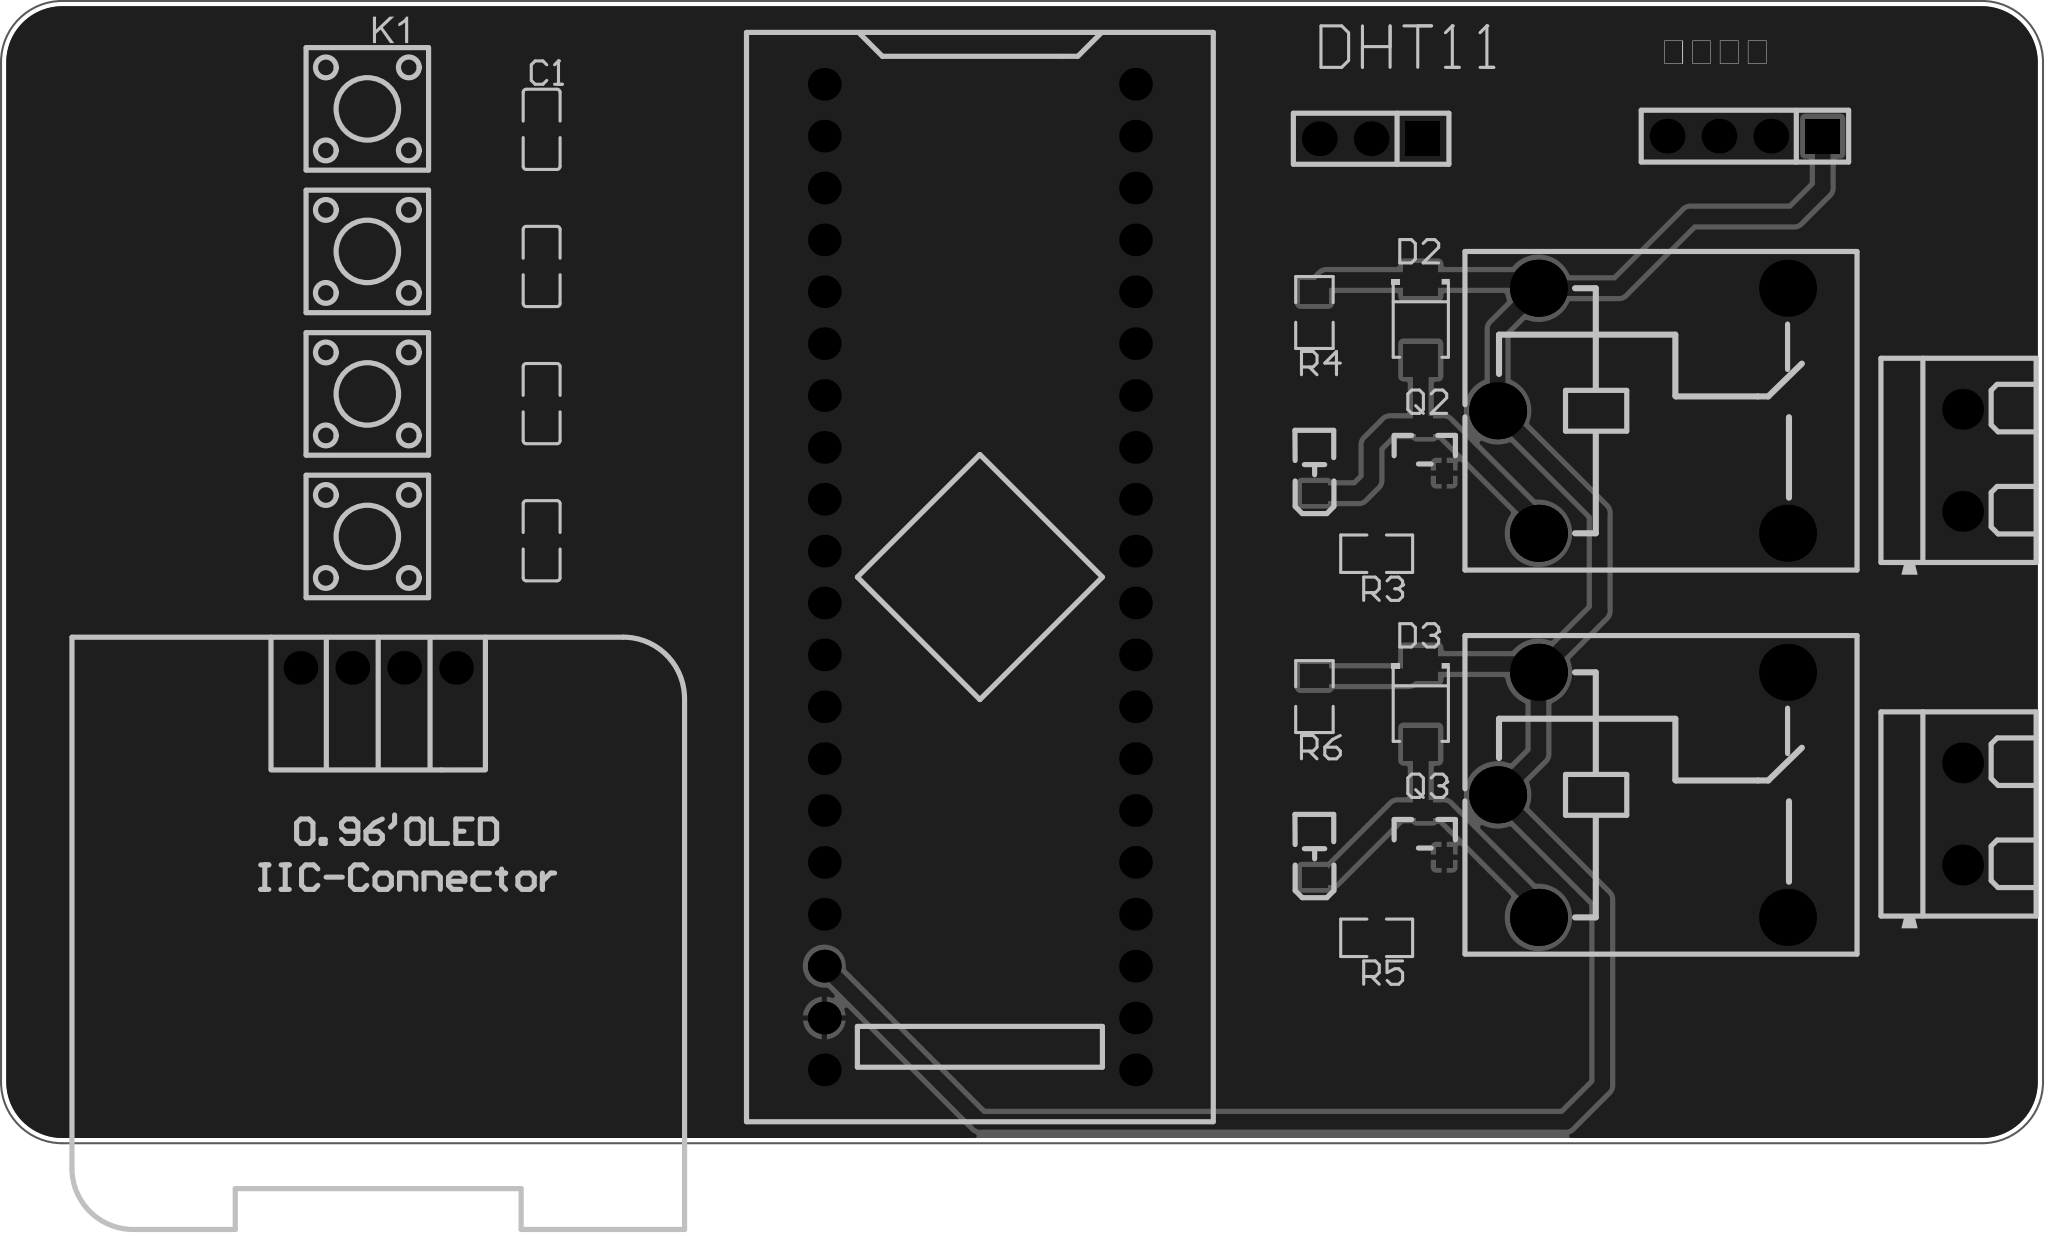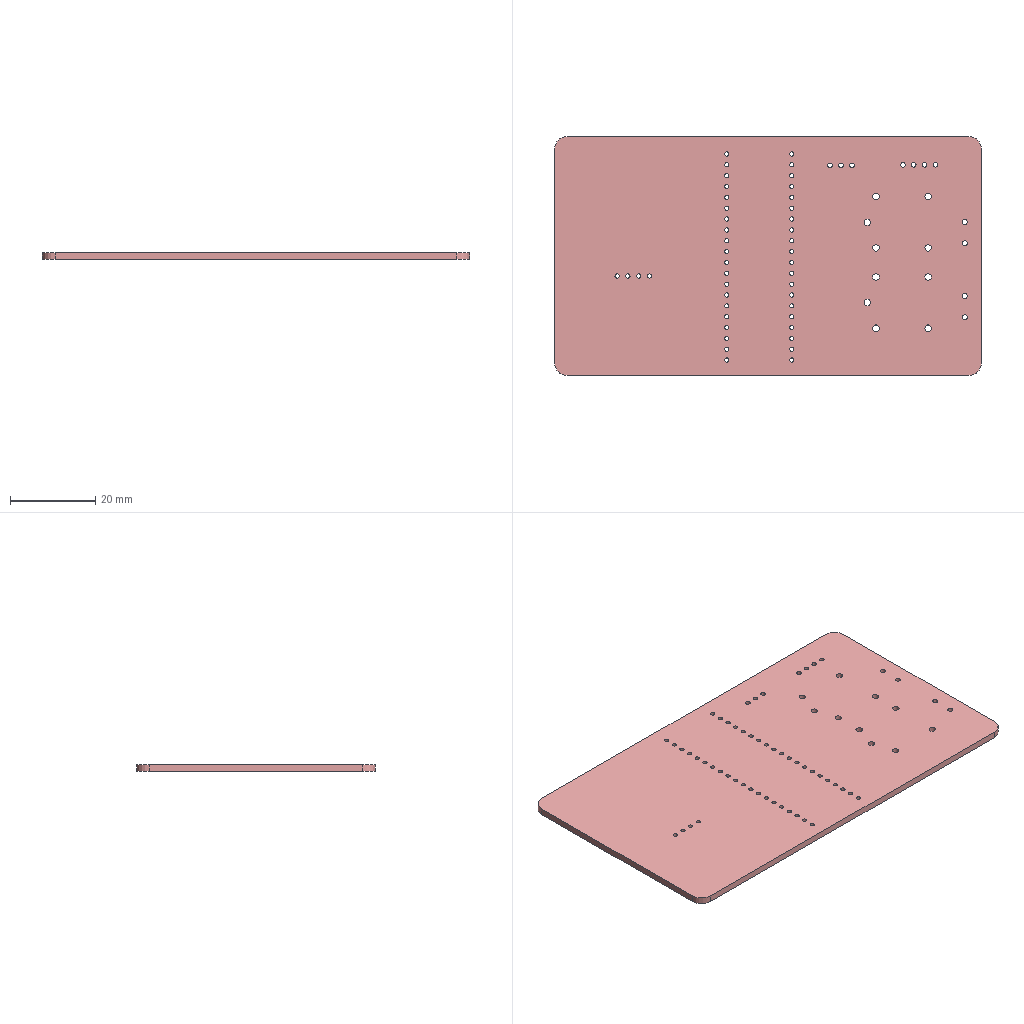Circuit board layout | Altium Designer | box 100 x 55.9 x 1.6 mm
Layer stack:
# Altium Designer layer stack of  (unit mm; dielectric type: 0 none, 1 core, 2 prepreg, 3 surface material)
index,name,kind,layer,copper_thickness_mm,dielectric_type,dielectric_thickness_mm,dielectric_material,dielectric_constant
0,Top Paste Mask Layer,other,,,,,,
1,Top Silkscreen Layer,other,,,,,,
2,Top Solder Mask Layer,dielectric,,,3,0.01,,3.3
3,Top Layer,copper,Top Layer,0.035,,,,
4,Dielectric1,dielectric,,,3,1.51,FR4,4.5
5,Bottom Layer,copper,Bottom Layer,0.035,,,,
6,Bottom Solder Mask Layer,dielectric,,,3,0.01,,3.3
7,Bottom Silkscreen Layer,other,,,,,,
8,Bottom Paste Mask Layer,other,,,,,,
# drill layer pairs: low layer,high layer
drill_pair,Top Layer,Bottom Layer
Part placement:
Designator,Comment,Layer,Footprint,Center-X(mm),Center-Y(mm),Rotation
U1,LCKFB-DKX-STM32F103C8T6,TopLayer,CONN-TH_L53.3-W22.9_STM32F103C8T6-CARD,124.137,108.245,270
K1,,TopLayer,SW-SMD_4P-L6.0-W6.0-P4.50-LS9.0-2,94.138,131.169,0
K2,,TopLayer,SW-SMD_4P-L6.0-W6.0-P4.50-LS9.0-2,94.138,124.191,0
K3,,TopLayer,SW-SMD_4P-L6.0-W6.0-P4.50-LS9.0-2,94.138,117.212,0
K4,,TopLayer,SW-SMD_4P-L6.0-W6.0-P4.50-LS9.0-2,94.138,110.234,0
D2,M7F,TopLayer,SMAF_L3.5-W2.6-LS4.7-RD,145.728,120.833,270
D3,M7F,TopLayer,SMAF_L3.5-W2.6-LS4.7-RD,145.728,102.027,270
K5,SRD-DC5V-SL-C,TopLayer,RELAY-TH_SRD-DCXXV-SL-C,156.591,116.388,0
K6,SRD-DC5V-SL-C,TopLayer,RELAY-TH_SRD-DCXXV-SL-C,156.591,97.582,0
OLED1,,TopLayer,0.96OLED_4P,94.673,103.8,0
Q2,,TopLayer,S8050_SOT-23,145.923,114.483,270
Q3,,TopLayer,S8050_SOT-23,145.923,95.677,270
P1,KF301-2P接线端子,TopLayer,CONN-TH_XY301V-A-5.0-2P,172.263,96.645,270
C1,100nF,TopLayer,C0805,102.674,130.169,270
C2,100nF,TopLayer,C0805,102.674,123.454,270
C3,100nF,TopLayer,C0805,102.674,116.738,270
C4,100nF,TopLayer,C0805,102.674,110.023,270
R3,330,TopLayer,R0805,143.568,109.388,180
R4,10K,TopLayer,R0805,140.52,121.199,90
R5,330,TopLayer,R0805,143.568,90.582,180
R6,10K,TopLayer,R0805,140.52,102.393,90
LED2,MS-PTV1608NWAF-B02,TopLayer,LED0805-RD_BLUE,140.525,113.452,90
LED3,MS-PTV1608NWAF-B02,TopLayer,LED0805-RD_BLUE,140.525,94.646,90
P3,KF301-2P接线端子,TopLayer,CONN-TH_XY301V-A-5.0-2P,172.263,113.96,270
DHT11,,TopLayer,HDR-TH_3P-P2.54-V-M,143.297,129.708,180
土壤湿度,,TopLayer,HDR-TH_4P-P2.54-V-M,161.602,129.835,180
Pad and via stacks:
# Altium Designer via and pad stacks of  (unit mm). Each distinct definition once, with the count of objects using it.
# via: kind,start_layer,end_layer,hole_mm,diameter_mm,mode(0 simple;1 top-mid-bottom;2 full stack),diameter_per_layer,count,example_net
# pad: kind,layer,hole_mm,hole_type(0 round;1 square;2 slot),plating,top_size,top_shape(1 round;2 rect;3 octagon;9 rounded rect),mid_size,bottom_size,mode,footprint,size_per_layer,count,example
pad,Multi-Layer,1,0,plated,1.6x1.6,1,1.6x1.6,1.6x1.6,0,CONN-TH_L53.3-W22.9_STM32F103C8T6-CARD,,40,U1.1
pad,Multi-Layer,1.524,0,plated,2.794x2.794,1,2.794x2.794,2.794x2.794,0,RELAY-TH_SRD-DCXXV-SL-C,,10,K5.2
pad,Multi-Layer,1,0,plated,1.65x1.65,1,1.65x1.65,1.65x1.65,0,0.96OLED_4P,,4,OLED1.4
pad,Multi-Layer,1.2,0,plated,2x2,1,2x2,2x2,0,CONN-TH_XY301V-A-5.0-2P,,4,P1.1
pad,Multi-Layer,1.1,0,plated,1.7x1.7,2,1.7x1.7,1.7x1.7,0,HDR-TH_3P-P2.54-V-M,,1,DHT11.1
pad,Multi-Layer,1.1,0,plated,1.7x1.7,1,1.7x1.7,1.7x1.7,0,HDR-TH_3P-P2.54-V-M,,2,DHT11.2
pad,Multi-Layer,1.1,0,plated,1.7x1.7,2,1.7x1.7,1.7x1.7,0,HDR-TH_4P-P2.54-V-M,,1,\u571F\u58E4\u6E7F\u5EA6.1
pad,Multi-Layer,1.1,0,plated,1.7x1.7,1,1.7x1.7,1.7x1.7,0,HDR-TH_4P-P2.54-V-M,,3,\u571F\u58E4\u6E7F\u5EA6.2
pad,Top Layer,0,0,plated,2.3x1.5,2,2.3x1.5,2.3x1.5,0,SW-SMD_4P-L6.0-W6.0-P4.50-LS9.0-2,,16,K1.1
pad,Top Layer,0,0,plated,1.6x1.7,2,1.6x1.7,1.6x1.7,0,SMAF_L3.5-W2.6-LS4.7-RD,,4,D2.2
pad,Top Layer,0,0,plated,1x0.8,2,1x0.8,1x0.8,0,S8050_SOT-23,,6,Q2.2
pad,Top Layer,0,0,plated,1.41x1.35,2,1.41x1.35,1.41x1.35,0,C0805,,8,C1.2
pad,Top Layer,0,0,plated,1.133x1.377,2,1.133x1.377,1.133x1.377,0,R0805,,8,R3.2
pad,Top Layer,0,0,plated,1x1.25,2,1x1.25,1x1.25,0,LED0805-RD_BLUE,,4,LED2.1
Copper pours:
name,layer,net,type(0 solid;1 hatched;2 none)
Top Layer-GND,Top Layer,GND,0
Bottom Layer-GND,Bottom Layer,GND,0